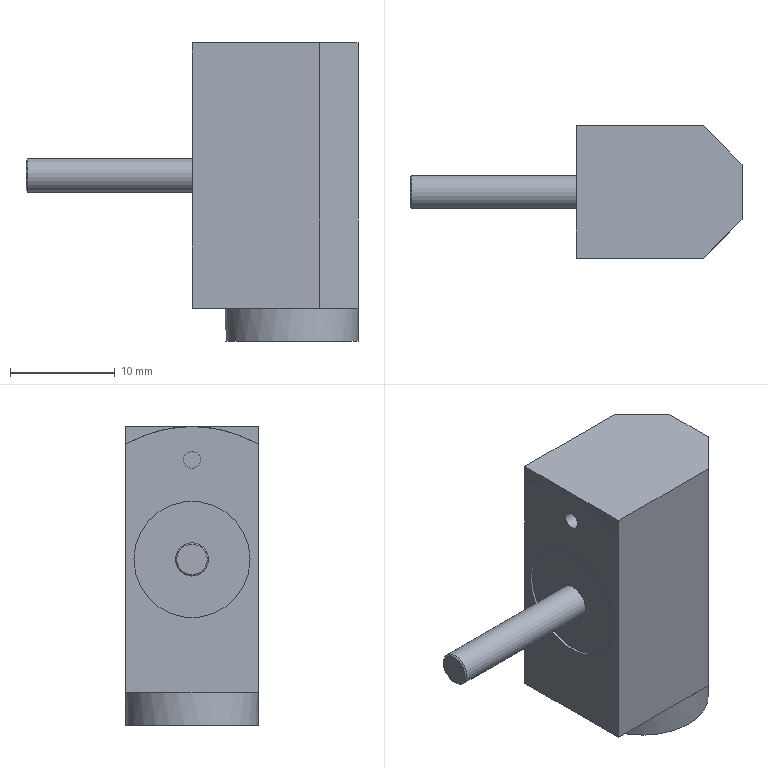Part | NX | features DATUM_CSYS 7, SKETCH 6, EXTRUDE 4, CYLINDER 2, CHAMFER 1, SWP104 1 | 1 solid | 26 faces | box 31.75 x 12.7 x 28.575 mm | volume 3399 mm3 | plane 19 | cylinder 6 | cone 1 | commonest cylinder face diameters 1.587 x1 3.175 x1 9.525 x1 11.113 x1 12.7 x1 25.4 x1
STEP:
#1=CARTESIAN_POINT('',(-9.271,-5.556,15.875));
#2=VERTEX_POINT('',#1);
#3=CARTESIAN_POINT('',(-9.271,0.,15.875));
#4=DIRECTION('',(-1.,0.,0.));
#5=DIRECTION('',(0.,-1.,0.));
#6=AXIS2_PLACEMENT_3D('',#3,#4,#5);
#7=CIRCLE('',#6,5.556);
#8=EDGE_CURVE('',#2,#2,#7,.F.);
#9=ORIENTED_EDGE('',*,*,#8,.F.);
#10=EDGE_LOOP('',(#9));
#11=FACE_BOUND('',#10,.T.);
#12=CARTESIAN_POINT('',(-9.271,0.,17.462));
#13=VERTEX_POINT('',#12);
#14=CARTESIAN_POINT('',(-9.271,0.,15.875));
#15=DIRECTION('',(-1.,0.,0.));
#16=DIRECTION('',(0.,0.,1.));
#17=AXIS2_PLACEMENT_3D('',#14,#15,#16);
#18=CIRCLE('',#17,1.587);
#19=EDGE_CURVE('',#13,#13,#18,.F.);
#20=ORIENTED_EDGE('',*,*,#19,.T.);
#21=EDGE_LOOP('',(#20));
#22=FACE_BOUND('',#21,.T.);
#23=CARTESIAN_POINT('',(-9.271,0.,15.875));
#24=DIRECTION('',(-1.,0.,0.));
#25=DIRECTION('',(0.,0.,1.));
#26=AXIS2_PLACEMENT_3D('',#23,#24,#25);
#27=PLANE('',#26);
#28=ADVANCED_FACE('',(#11,#22),#27,.T.);
#29=CARTESIAN_POINT('',(6.35,0.,0.));
#30=VERTEX_POINT('',#29);
#31=CARTESIAN_POINT('',(0.,0.,0.));
#32=DIRECTION('',(0.,0.,1.));
#33=DIRECTION('',(1.,0.,0.));
#34=AXIS2_PLACEMENT_3D('',#31,#32,#33);
#35=CIRCLE('',#34,6.35);
#36=EDGE_CURVE('',#30,#30,#35,.T.);
#37=ORIENTED_EDGE('',*,*,#36,.T.);
#38=EDGE_LOOP('',(#37));
#39=FACE_BOUND('',#38,.T.);
#40=CARTESIAN_POINT('',(4.49,4.49,3.175));
#41=VERTEX_POINT('',#40);
#42=CARTESIAN_POINT('',(6.35,0.,3.175));
#43=VERTEX_POINT('',#42);
#44=CARTESIAN_POINT('',(0.,0.,3.175));
#45=DIRECTION('',(0.,0.,1.));
#46=DIRECTION('',(1.,0.,0.));
#47=AXIS2_PLACEMENT_3D('',#44,#45,#46);
#48=CIRCLE('',#47,6.35);
#49=EDGE_CURVE('',#41,#43,#48,.F.);
#50=ORIENTED_EDGE('',*,*,#49,.T.);
#51=CARTESIAN_POINT('',(4.49,-4.49,3.175));
#52=VERTEX_POINT('',#51);
#53=CARTESIAN_POINT('',(0.,0.,3.175));
#54=DIRECTION('',(0.,0.,1.));
#55=DIRECTION('',(1.,0.,0.));
#56=AXIS2_PLACEMENT_3D('',#53,#54,#55);
#57=CIRCLE('',#56,6.35);
#58=EDGE_CURVE('',#43,#52,#57,.F.);
#59=ORIENTED_EDGE('',*,*,#58,.T.);
#60=CARTESIAN_POINT('',(0.,-6.35,3.175));
#61=VERTEX_POINT('',#60);
#62=CARTESIAN_POINT('',(0.,0.,3.175));
#63=DIRECTION('',(0.,0.,1.));
#64=DIRECTION('',(1.,0.,0.));
#65=AXIS2_PLACEMENT_3D('',#62,#63,#64);
#66=CIRCLE('',#65,6.35);
#67=EDGE_CURVE('',#52,#61,#66,.F.);
#68=ORIENTED_EDGE('',*,*,#67,.T.);
#69=CARTESIAN_POINT('',(0.,6.35,3.175));
#70=VERTEX_POINT('',#69);
#71=CARTESIAN_POINT('',(0.,0.,3.175));
#72=DIRECTION('',(0.,0.,1.));
#73=DIRECTION('',(1.,0.,0.));
#74=AXIS2_PLACEMENT_3D('',#71,#72,#73);
#75=CIRCLE('',#74,6.35);
#76=EDGE_CURVE('',#61,#70,#75,.F.);
#77=ORIENTED_EDGE('',*,*,#76,.T.);
#78=CARTESIAN_POINT('',(0.,0.,3.175));
#79=DIRECTION('',(0.,0.,1.));
#80=DIRECTION('',(1.,0.,0.));
#81=AXIS2_PLACEMENT_3D('',#78,#79,#80);
#82=CIRCLE('',#81,6.35);
#83=EDGE_CURVE('',#70,#41,#82,.F.);
#84=ORIENTED_EDGE('',*,*,#83,.T.);
#85=EDGE_LOOP('',(#50,#59,#68,#77,#84));
#86=FACE_BOUND('',#85,.T.);
#87=CARTESIAN_POINT('',(0.,0.,0.));
#88=DIRECTION('',(0.,0.,1.));
#89=DIRECTION('',(1.,0.,0.));
#90=AXIS2_PLACEMENT_3D('',#87,#88,#89);
#91=CYLINDRICAL_SURFACE('',#90,6.35);
#92=ADVANCED_FACE('',(#39,#86),#91,.T.);
#93=CARTESIAN_POINT('',(4.763,0.,0.));
#94=VERTEX_POINT('',#93);
#95=CARTESIAN_POINT('',(0.,0.,0.));
#96=DIRECTION('',(0.,0.,1.));
#97=DIRECTION('',(1.,0.,0.));
#98=AXIS2_PLACEMENT_3D('',#95,#96,#97);
#99=CIRCLE('',#98,4.763);
#100=EDGE_CURVE('',#94,#94,#99,.T.);
#101=ORIENTED_EDGE('',*,*,#100,.T.);
#102=EDGE_LOOP('',(#101));
#103=FACE_BOUND('',#102,.T.);
#104=ORIENTED_EDGE('',*,*,#36,.F.);
#105=EDGE_LOOP('',(#104));
#106=FACE_BOUND('',#105,.T.);
#107=CARTESIAN_POINT('',(0.,0.,0.));
#108=DIRECTION('',(0.,0.,-1.));
#109=DIRECTION('',(-1.,0.,0.));
#110=AXIS2_PLACEMENT_3D('',#107,#108,#109);
#111=PLANE('',#110);
#112=ADVANCED_FACE('',(#103,#106),#111,.T.);
#113=CARTESIAN_POINT('',(-9.52,-6.35,28.575));
#114=VERTEX_POINT('',#113);
#115=CARTESIAN_POINT('',(-9.52,-6.35,26.874));
#116=VERTEX_POINT('',#115);
#117=CARTESIAN_POINT('',(-9.52,-6.35,282.892));
#118=DIRECTION('',(0.,0.,-1.));
#119=VECTOR('',#118,1000.);
#120=LINE('',#117,#119);
#121=EDGE_CURVE('',#114,#116,#120,.T.);
#122=ORIENTED_EDGE('',*,*,#121,.T.);
#123=CARTESIAN_POINT('',(-9.525,-6.35,26.874));
#124=VERTEX_POINT('',#123);
#125=CARTESIAN_POINT('',(-9.52,-6.35,26.874));
#126=DIRECTION('',(-1.,0.,0.));
#127=VECTOR('',#126,1000.);
#128=LINE('',#125,#127);
#129=EDGE_CURVE('',#116,#124,#128,.T.);
#130=ORIENTED_EDGE('',*,*,#129,.T.);
#131=CARTESIAN_POINT('',(-9.525,-6.35,3.175));
#132=VERTEX_POINT('',#131);
#133=CARTESIAN_POINT('',(-9.525,-6.35,282.892));
#134=DIRECTION('',(0.,0.,-1.));
#135=VECTOR('',#134,1000.);
#136=LINE('',#133,#135);
#137=EDGE_CURVE('',#124,#132,#136,.T.);
#138=ORIENTED_EDGE('',*,*,#137,.T.);
#139=CARTESIAN_POINT('',(-9.525,-6.35,3.175));
#140=DIRECTION('',(1.,0.,0.));
#141=VECTOR('',#140,1000.);
#142=LINE('',#139,#141);
#143=EDGE_CURVE('',#132,#61,#142,.T.);
#144=ORIENTED_EDGE('',*,*,#143,.T.);
#145=CARTESIAN_POINT('',(2.63,-6.35,3.175));
#146=VERTEX_POINT('',#145);
#147=CARTESIAN_POINT('',(-9.525,-6.35,3.175));
#148=DIRECTION('',(1.,0.,0.));
#149=VECTOR('',#148,1000.);
#150=LINE('',#147,#149);
#151=EDGE_CURVE('',#61,#146,#150,.T.);
#152=ORIENTED_EDGE('',*,*,#151,.T.);
#153=CARTESIAN_POINT('',(2.63,-6.35,28.575));
#154=VERTEX_POINT('',#153);
#155=CARTESIAN_POINT('',(2.63,-6.35,282.892));
#156=DIRECTION('',(0.,0.,-1.));
#157=VECTOR('',#156,1000.);
#158=LINE('',#155,#157);
#159=EDGE_CURVE('',#154,#146,#158,.T.);
#160=ORIENTED_EDGE('',*,*,#159,.F.);
#161=CARTESIAN_POINT('',(-9.525,-6.35,28.575));
#162=DIRECTION('',(1.,0.,0.));
#163=VECTOR('',#162,1000.);
#164=LINE('',#161,#163);
#165=EDGE_CURVE('',#114,#154,#164,.T.);
#166=ORIENTED_EDGE('',*,*,#165,.F.);
#167=EDGE_LOOP('',(#122,#130,#138,#144,#152,#160,#166));
#168=FACE_BOUND('',#167,.T.);
#169=CARTESIAN_POINT('',(-9.525,-6.35,282.892));
#170=DIRECTION('',(0.,1.,0.));
#171=DIRECTION('',(-1.,0.,0.));
#172=AXIS2_PLACEMENT_3D('',#169,#170,#171);
#173=PLANE('',#172);
#174=ADVANCED_FACE('',(#168),#173,.F.);
#175=CARTESIAN_POINT('',(6.35,-2.63,28.575));
#176=VERTEX_POINT('',#175);
#177=CARTESIAN_POINT('',(2.63,-6.35,28.575));
#178=DIRECTION('',(0.7071,0.7071,0.));
#179=VECTOR('',#178,1000.);
#180=LINE('',#177,#179);
#181=EDGE_CURVE('',#154,#176,#180,.T.);
#182=ORIENTED_EDGE('',*,*,#181,.F.);
#183=ORIENTED_EDGE('',*,*,#159,.T.);
#184=CARTESIAN_POINT('',(2.63,-6.35,3.175));
#185=DIRECTION('',(0.7071,0.7071,0.));
#186=VECTOR('',#185,1000.);
#187=LINE('',#184,#186);
#188=EDGE_CURVE('',#146,#52,#187,.T.);
#189=ORIENTED_EDGE('',*,*,#188,.T.);
#190=CARTESIAN_POINT('',(6.35,-2.63,3.175));
#191=VERTEX_POINT('',#190);
#192=CARTESIAN_POINT('',(2.63,-6.35,3.175));
#193=DIRECTION('',(0.7071,0.7071,0.));
#194=VECTOR('',#193,1000.);
#195=LINE('',#192,#194);
#196=EDGE_CURVE('',#52,#191,#195,.T.);
#197=ORIENTED_EDGE('',*,*,#196,.T.);
#198=CARTESIAN_POINT('',(6.35,-2.63,282.892));
#199=DIRECTION('',(0.,0.,-1.));
#200=VECTOR('',#199,1000.);
#201=LINE('',#198,#200);
#202=EDGE_CURVE('',#176,#191,#201,.T.);
#203=ORIENTED_EDGE('',*,*,#202,.F.);
#204=EDGE_LOOP('',(#182,#183,#189,#197,#203));
#205=FACE_BOUND('',#204,.T.);
#206=CARTESIAN_POINT('',(2.63,-6.35,282.892));
#207=DIRECTION('',(-0.7071,0.7071,0.));
#208=DIRECTION('',(-0.7071,-0.7071,0.));
#209=AXIS2_PLACEMENT_3D('',#206,#207,#208);
#210=PLANE('',#209);
#211=ADVANCED_FACE('',(#205),#210,.F.);
#212=CARTESIAN_POINT('',(6.35,2.63,28.575));
#213=VERTEX_POINT('',#212);
#214=CARTESIAN_POINT('',(6.35,2.63,3.175));
#215=VERTEX_POINT('',#214);
#216=CARTESIAN_POINT('',(6.35,2.63,282.892));
#217=DIRECTION('',(0.,0.,-1.));
#218=VECTOR('',#217,1000.);
#219=LINE('',#216,#218);
#220=EDGE_CURVE('',#213,#215,#219,.T.);
#221=ORIENTED_EDGE('',*,*,#220,.F.);
#222=CARTESIAN_POINT('',(6.35,-2.63,28.575));
#223=DIRECTION('',(0.,1.,0.));
#224=VECTOR('',#223,1000.);
#225=LINE('',#222,#224);
#226=EDGE_CURVE('',#176,#213,#225,.T.);
#227=ORIENTED_EDGE('',*,*,#226,.F.);
#228=ORIENTED_EDGE('',*,*,#202,.T.);
#229=CARTESIAN_POINT('',(6.35,-2.63,3.175));
#230=DIRECTION('',(0.,1.,0.));
#231=VECTOR('',#230,1000.);
#232=LINE('',#229,#231);
#233=EDGE_CURVE('',#191,#43,#232,.T.);
#234=ORIENTED_EDGE('',*,*,#233,.T.);
#235=CARTESIAN_POINT('',(6.35,-2.63,3.175));
#236=DIRECTION('',(0.,1.,0.));
#237=VECTOR('',#236,1000.);
#238=LINE('',#235,#237);
#239=EDGE_CURVE('',#43,#215,#238,.T.);
#240=ORIENTED_EDGE('',*,*,#239,.T.);
#241=EDGE_LOOP('',(#221,#227,#228,#234,#240));
#242=FACE_BOUND('',#241,.T.);
#243=CARTESIAN_POINT('',(6.35,-2.63,282.892));
#244=DIRECTION('',(-1.,0.,0.));
#245=DIRECTION('',(0.,-1.,0.));
#246=AXIS2_PLACEMENT_3D('',#243,#244,#245);
#247=PLANE('',#246);
#248=ADVANCED_FACE('',(#242),#247,.F.);
#249=CARTESIAN_POINT('',(2.63,6.35,28.575));
#250=VERTEX_POINT('',#249);
#251=CARTESIAN_POINT('',(6.35,2.63,28.575));
#252=DIRECTION('',(-0.7071,0.7071,0.));
#253=VECTOR('',#252,1000.);
#254=LINE('',#251,#253);
#255=EDGE_CURVE('',#213,#250,#254,.T.);
#256=ORIENTED_EDGE('',*,*,#255,.F.);
#257=ORIENTED_EDGE('',*,*,#220,.T.);
#258=CARTESIAN_POINT('',(6.35,2.63,3.175));
#259=DIRECTION('',(-0.7071,0.7071,0.));
#260=VECTOR('',#259,1000.);
#261=LINE('',#258,#260);
#262=EDGE_CURVE('',#215,#41,#261,.T.);
#263=ORIENTED_EDGE('',*,*,#262,.T.);
#264=CARTESIAN_POINT('',(2.63,6.35,3.175));
#265=VERTEX_POINT('',#264);
#266=CARTESIAN_POINT('',(6.35,2.63,3.175));
#267=DIRECTION('',(-0.7071,0.7071,0.));
#268=VECTOR('',#267,1000.);
#269=LINE('',#266,#268);
#270=EDGE_CURVE('',#41,#265,#269,.T.);
#271=ORIENTED_EDGE('',*,*,#270,.T.);
#272=CARTESIAN_POINT('',(2.63,6.35,282.892));
#273=DIRECTION('',(0.,0.,-1.));
#274=VECTOR('',#273,1000.);
#275=LINE('',#272,#274);
#276=EDGE_CURVE('',#250,#265,#275,.T.);
#277=ORIENTED_EDGE('',*,*,#276,.F.);
#278=EDGE_LOOP('',(#256,#257,#263,#271,#277));
#279=FACE_BOUND('',#278,.T.);
#280=CARTESIAN_POINT('',(6.35,2.63,282.892));
#281=DIRECTION('',(-0.7071,-0.7071,0.));
#282=DIRECTION('',(0.7071,-0.7071,0.));
#283=AXIS2_PLACEMENT_3D('',#280,#281,#282);
#284=PLANE('',#283);
#285=ADVANCED_FACE('',(#279),#284,.F.);
#286=CARTESIAN_POINT('',(-9.525,6.35,26.874));
#287=VERTEX_POINT('',#286);
#288=CARTESIAN_POINT('',(-9.525,6.35,3.175));
#289=VERTEX_POINT('',#288);
#290=CARTESIAN_POINT('',(-9.525,6.35,282.892));
#291=DIRECTION('',(0.,0.,-1.));
#292=VECTOR('',#291,1000.);
#293=LINE('',#290,#292);
#294=EDGE_CURVE('',#287,#289,#293,.T.);
#295=ORIENTED_EDGE('',*,*,#294,.F.);
#296=CARTESIAN_POINT('',(-9.52,6.35,26.874));
#297=VERTEX_POINT('',#296);
#298=CARTESIAN_POINT('',(-9.52,6.35,26.874));
#299=DIRECTION('',(-1.,0.,0.));
#300=VECTOR('',#299,1000.);
#301=LINE('',#298,#300);
#302=EDGE_CURVE('',#287,#297,#301,.F.);
#303=ORIENTED_EDGE('',*,*,#302,.T.);
#304=CARTESIAN_POINT('',(-9.52,6.35,28.575));
#305=VERTEX_POINT('',#304);
#306=CARTESIAN_POINT('',(-9.52,6.35,282.892));
#307=DIRECTION('',(0.,0.,1.));
#308=VECTOR('',#307,1000.);
#309=LINE('',#306,#308);
#310=EDGE_CURVE('',#297,#305,#309,.T.);
#311=ORIENTED_EDGE('',*,*,#310,.T.);
#312=CARTESIAN_POINT('',(2.63,6.35,28.575));
#313=DIRECTION('',(-1.,0.,0.));
#314=VECTOR('',#313,1000.);
#315=LINE('',#312,#314);
#316=EDGE_CURVE('',#250,#305,#315,.T.);
#317=ORIENTED_EDGE('',*,*,#316,.F.);
#318=ORIENTED_EDGE('',*,*,#276,.T.);
#319=CARTESIAN_POINT('',(2.63,6.35,3.175));
#320=DIRECTION('',(-1.,0.,0.));
#321=VECTOR('',#320,1000.);
#322=LINE('',#319,#321);
#323=EDGE_CURVE('',#265,#70,#322,.T.);
#324=ORIENTED_EDGE('',*,*,#323,.T.);
#325=CARTESIAN_POINT('',(2.63,6.35,3.175));
#326=DIRECTION('',(-1.,0.,0.));
#327=VECTOR('',#326,1000.);
#328=LINE('',#325,#327);
#329=EDGE_CURVE('',#70,#289,#328,.T.);
#330=ORIENTED_EDGE('',*,*,#329,.T.);
#331=EDGE_LOOP('',(#295,#303,#311,#317,#318,#324,#330));
#332=FACE_BOUND('',#331,.T.);
#333=CARTESIAN_POINT('',(2.63,6.35,282.892));
#334=DIRECTION('',(0.,-1.,0.));
#335=DIRECTION('',(0.,0.,-1.));
#336=AXIS2_PLACEMENT_3D('',#333,#334,#335);
#337=PLANE('',#336);
#338=ADVANCED_FACE('',(#332),#337,.F.);
#339=ORIENTED_EDGE('',*,*,#58,.F.);
#340=ORIENTED_EDGE('',*,*,#233,.F.);
#341=ORIENTED_EDGE('',*,*,#196,.F.);
#342=EDGE_LOOP('',(#339,#340,#341));
#343=FACE_BOUND('',#342,.T.);
#344=CARTESIAN_POINT('',(0.,0.,3.175));
#345=DIRECTION('',(0.,0.,1.));
#346=DIRECTION('',(1.,0.,0.));
#347=AXIS2_PLACEMENT_3D('',#344,#345,#346);
#348=PLANE('',#347);
#349=ADVANCED_FACE('',(#343),#348,.F.);
#350=ORIENTED_EDGE('',*,*,#67,.F.);
#351=ORIENTED_EDGE('',*,*,#188,.F.);
#352=ORIENTED_EDGE('',*,*,#151,.F.);
#353=EDGE_LOOP('',(#350,#351,#352));
#354=FACE_BOUND('',#353,.T.);
#355=CARTESIAN_POINT('',(0.,0.,3.175));
#356=DIRECTION('',(0.,0.,1.));
#357=DIRECTION('',(1.,0.,0.));
#358=AXIS2_PLACEMENT_3D('',#355,#356,#357);
#359=PLANE('',#358);
#360=ADVANCED_FACE('',(#354),#359,.F.);
#361=ORIENTED_EDGE('',*,*,#76,.F.);
#362=ORIENTED_EDGE('',*,*,#143,.F.);
#363=CARTESIAN_POINT('',(-9.525,6.35,3.175));
#364=DIRECTION('',(0.,-1.,0.));
#365=VECTOR('',#364,1000.);
#366=LINE('',#363,#365);
#367=EDGE_CURVE('',#289,#132,#366,.T.);
#368=ORIENTED_EDGE('',*,*,#367,.F.);
#369=ORIENTED_EDGE('',*,*,#329,.F.);
#370=EDGE_LOOP('',(#361,#362,#368,#369));
#371=FACE_BOUND('',#370,.T.);
#372=CARTESIAN_POINT('',(0.,0.,3.175));
#373=DIRECTION('',(0.,0.,1.));
#374=DIRECTION('',(1.,0.,0.));
#375=AXIS2_PLACEMENT_3D('',#372,#373,#374);
#376=PLANE('',#375);
#377=ADVANCED_FACE('',(#371),#376,.F.);
#378=ORIENTED_EDGE('',*,*,#83,.F.);
#379=ORIENTED_EDGE('',*,*,#323,.F.);
#380=ORIENTED_EDGE('',*,*,#270,.F.);
#381=EDGE_LOOP('',(#378,#379,#380));
#382=FACE_BOUND('',#381,.T.);
#383=CARTESIAN_POINT('',(0.,0.,3.175));
#384=DIRECTION('',(0.,0.,1.));
#385=DIRECTION('',(1.,0.,0.));
#386=AXIS2_PLACEMENT_3D('',#383,#384,#385);
#387=PLANE('',#386);
#388=ADVANCED_FACE('',(#382),#387,.F.);
#389=CARTESIAN_POINT('',(-9.525,-5.556,15.875));
#390=VERTEX_POINT('',#389);
#391=CARTESIAN_POINT('',(-9.525,0.,15.875));
#392=DIRECTION('',(-1.,0.,0.));
#393=DIRECTION('',(0.,-1.,0.));
#394=AXIS2_PLACEMENT_3D('',#391,#392,#393);
#395=CIRCLE('',#394,5.556);
#396=EDGE_CURVE('',#390,#390,#395,.T.);
#397=ORIENTED_EDGE('',*,*,#396,.F.);
#398=EDGE_LOOP('',(#397));
#399=FACE_BOUND('',#398,.T.);
#400=CARTESIAN_POINT('',(-9.525,-0.7937,25.4));
#401=VERTEX_POINT('',#400);
#402=CARTESIAN_POINT('',(-9.525,0.,25.4));
#403=DIRECTION('',(-1.,0.,0.));
#404=DIRECTION('',(0.,-1.,0.));
#405=AXIS2_PLACEMENT_3D('',#402,#403,#404);
#406=CIRCLE('',#405,0.7937);
#407=EDGE_CURVE('',#401,#401,#406,.T.);
#408=ORIENTED_EDGE('',*,*,#407,.F.);
#409=EDGE_LOOP('',(#408));
#410=FACE_BOUND('',#409,.T.);
#411=CARTESIAN_POINT('',(-9.525,0.,15.875));
#412=DIRECTION('',(1.,0.,0.));
#413=DIRECTION('',(0.,-1.,0.));
#414=AXIS2_PLACEMENT_3D('',#411,#412,#413);
#415=CIRCLE('',#414,12.7);
#416=EDGE_CURVE('',#287,#124,#415,.T.);
#417=ORIENTED_EDGE('',*,*,#416,.F.);
#418=ORIENTED_EDGE('',*,*,#294,.T.);
#419=ORIENTED_EDGE('',*,*,#367,.T.);
#420=ORIENTED_EDGE('',*,*,#137,.F.);
#421=EDGE_LOOP('',(#417,#418,#419,#420));
#422=FACE_BOUND('',#421,.T.);
#423=CARTESIAN_POINT('',(-9.525,6.35,282.892));
#424=DIRECTION('',(1.,0.,0.));
#425=DIRECTION('',(0.,1.,0.));
#426=AXIS2_PLACEMENT_3D('',#423,#424,#425);
#427=PLANE('',#426);
#428=ADVANCED_FACE('',(#399,#410,#422),#427,.F.);
#429=ORIENTED_EDGE('',*,*,#49,.F.);
#430=ORIENTED_EDGE('',*,*,#262,.F.);
#431=ORIENTED_EDGE('',*,*,#239,.F.);
#432=EDGE_LOOP('',(#429,#430,#431));
#433=FACE_BOUND('',#432,.T.);
#434=CARTESIAN_POINT('',(0.,0.,3.175));
#435=DIRECTION('',(0.,0.,1.));
#436=DIRECTION('',(1.,0.,0.));
#437=AXIS2_PLACEMENT_3D('',#434,#435,#436);
#438=PLANE('',#437);
#439=ADVANCED_FACE('',(#433),#438,.F.);
#440=CARTESIAN_POINT('',(-9.52,0.,28.575));
#441=VERTEX_POINT('',#440);
#442=CARTESIAN_POINT('',(-9.52,0.,28.575));
#443=DIRECTION('',(0.,1.,0.));
#444=VECTOR('',#443,1000.);
#445=LINE('',#442,#444);
#446=EDGE_CURVE('',#114,#441,#445,.T.);
#447=ORIENTED_EDGE('',*,*,#446,.F.);
#448=ORIENTED_EDGE('',*,*,#165,.T.);
#449=ORIENTED_EDGE('',*,*,#181,.T.);
#450=ORIENTED_EDGE('',*,*,#226,.T.);
#451=ORIENTED_EDGE('',*,*,#255,.T.);
#452=ORIENTED_EDGE('',*,*,#316,.T.);
#453=CARTESIAN_POINT('',(-9.52,0.,28.575));
#454=DIRECTION('',(0.,1.,0.));
#455=VECTOR('',#454,1000.);
#456=LINE('',#453,#455);
#457=EDGE_CURVE('',#441,#305,#456,.T.);
#458=ORIENTED_EDGE('',*,*,#457,.F.);
#459=EDGE_LOOP('',(#447,#448,#449,#450,#451,#452,#458));
#460=FACE_BOUND('',#459,.T.);
#461=CARTESIAN_POINT('',(0.,0.,28.575));
#462=DIRECTION('',(0.,0.,1.));
#463=DIRECTION('',(1.,0.,0.));
#464=AXIS2_PLACEMENT_3D('',#461,#462,#463);
#465=PLANE('',#464);
#466=ADVANCED_FACE('',(#460),#465,.T.);
#467=CARTESIAN_POINT('',(-9.52,0.,15.875));
#468=DIRECTION('',(1.,0.,0.));
#469=DIRECTION('',(0.,-1.,0.));
#470=AXIS2_PLACEMENT_3D('',#467,#468,#469);
#471=CIRCLE('',#470,12.7);
#472=EDGE_CURVE('',#116,#441,#471,.F.);
#473=ORIENTED_EDGE('',*,*,#472,.T.);
#474=CARTESIAN_POINT('',(-9.52,0.,15.875));
#475=DIRECTION('',(1.,0.,0.));
#476=DIRECTION('',(0.,-1.,0.));
#477=AXIS2_PLACEMENT_3D('',#474,#475,#476);
#478=CIRCLE('',#477,12.7);
#479=EDGE_CURVE('',#441,#297,#478,.F.);
#480=ORIENTED_EDGE('',*,*,#479,.T.);
#481=ORIENTED_EDGE('',*,*,#302,.F.);
#482=ORIENTED_EDGE('',*,*,#416,.T.);
#483=ORIENTED_EDGE('',*,*,#129,.F.);
#484=EDGE_LOOP('',(#473,#480,#481,#482,#483));
#485=FACE_BOUND('',#484,.T.);
#486=CARTESIAN_POINT('',(-9.52,0.,15.875));
#487=DIRECTION('',(-1.,0.,0.));
#488=DIRECTION('',(0.,0.,1.));
#489=AXIS2_PLACEMENT_3D('',#486,#487,#488);
#490=CYLINDRICAL_SURFACE('',#489,12.7);
#491=ADVANCED_FACE('',(#485),#490,.T.);
#492=ORIENTED_EDGE('',*,*,#446,.T.);
#493=ORIENTED_EDGE('',*,*,#472,.F.);
#494=ORIENTED_EDGE('',*,*,#121,.F.);
#495=EDGE_LOOP('',(#492,#493,#494));
#496=FACE_BOUND('',#495,.T.);
#497=CARTESIAN_POINT('',(-9.52,0.,15.875));
#498=DIRECTION('',(1.,0.,0.));
#499=DIRECTION('',(0.,0.,-1.));
#500=AXIS2_PLACEMENT_3D('',#497,#498,#499);
#501=PLANE('',#500);
#502=ADVANCED_FACE('',(#496),#501,.F.);
#503=ORIENTED_EDGE('',*,*,#479,.F.);
#504=ORIENTED_EDGE('',*,*,#457,.T.);
#505=ORIENTED_EDGE('',*,*,#310,.F.);
#506=EDGE_LOOP('',(#503,#504,#505));
#507=FACE_BOUND('',#506,.T.);
#508=CARTESIAN_POINT('',(-9.52,0.,15.875));
#509=DIRECTION('',(1.,0.,0.));
#510=DIRECTION('',(0.,0.,-1.));
#511=AXIS2_PLACEMENT_3D('',#508,#509,#510);
#512=PLANE('',#511);
#513=ADVANCED_FACE('',(#507),#512,.F.);
#514=CARTESIAN_POINT('',(-4.953,-0.7937,25.4));
#515=VERTEX_POINT('',#514);
#516=CARTESIAN_POINT('',(-4.953,0.,25.4));
#517=DIRECTION('',(-1.,0.,0.));
#518=DIRECTION('',(0.,-1.,0.));
#519=AXIS2_PLACEMENT_3D('',#516,#517,#518);
#520=CIRCLE('',#519,0.7937);
#521=EDGE_CURVE('',#515,#515,#520,.F.);
#522=ORIENTED_EDGE('',*,*,#521,.T.);
#523=EDGE_LOOP('',(#522));
#524=FACE_BOUND('',#523,.T.);
#525=ORIENTED_EDGE('',*,*,#407,.T.);
#526=EDGE_LOOP('',(#525));
#527=FACE_BOUND('',#526,.T.);
#528=CARTESIAN_POINT('',(-4.953,0.,25.4));
#529=DIRECTION('',(-1.,0.,0.));
#530=DIRECTION('',(0.,-1.,0.));
#531=AXIS2_PLACEMENT_3D('',#528,#529,#530);
#532=CYLINDRICAL_SURFACE('',#531,0.7937);
#533=ADVANCED_FACE('',(#524,#527),#532,.F.);
#534=ORIENTED_EDGE('',*,*,#521,.F.);
#535=EDGE_LOOP('',(#534));
#536=FACE_BOUND('',#535,.T.);
#537=CARTESIAN_POINT('',(-4.953,0.,25.4));
#538=DIRECTION('',(-1.,0.,0.));
#539=DIRECTION('',(0.,0.,1.));
#540=AXIS2_PLACEMENT_3D('',#537,#538,#539);
#541=PLANE('',#540);
#542=ADVANCED_FACE('',(#536),#541,.T.);
#543=ORIENTED_EDGE('',*,*,#8,.T.);
#544=EDGE_LOOP('',(#543));
#545=FACE_BOUND('',#544,.T.);
#546=ORIENTED_EDGE('',*,*,#396,.T.);
#547=EDGE_LOOP('',(#546));
#548=FACE_BOUND('',#547,.T.);
#549=CARTESIAN_POINT('',(-9.271,0.,15.875));
#550=DIRECTION('',(-1.,0.,0.));
#551=DIRECTION('',(0.,0.,1.));
#552=AXIS2_PLACEMENT_3D('',#549,#550,#551);
#553=CYLINDRICAL_SURFACE('',#552,5.556);
#554=ADVANCED_FACE('',(#545,#548),#553,.F.);
#555=CARTESIAN_POINT('',(-25.273,0.,17.462));
#556=VERTEX_POINT('',#555);
#557=CARTESIAN_POINT('',(-25.273,0.,15.875));
#558=DIRECTION('',(-1.,0.,0.));
#559=DIRECTION('',(0.,0.,1.));
#560=AXIS2_PLACEMENT_3D('',#557,#558,#559);
#561=CIRCLE('',#560,1.587);
#562=EDGE_CURVE('',#556,#556,#561,.F.);
#563=ORIENTED_EDGE('',*,*,#562,.T.);
#564=EDGE_LOOP('',(#563));
#565=FACE_BOUND('',#564,.T.);
#566=ORIENTED_EDGE('',*,*,#19,.F.);
#567=EDGE_LOOP('',(#566));
#568=FACE_BOUND('',#567,.T.);
#569=CARTESIAN_POINT('',(-25.4,0.,15.875));
#570=DIRECTION('',(1.,0.,0.));
#571=DIRECTION('',(0.,0.,-1.));
#572=AXIS2_PLACEMENT_3D('',#569,#570,#571);
#573=CYLINDRICAL_SURFACE('',#572,1.587);
#574=ADVANCED_FACE('',(#565,#568),#573,.T.);
#575=CARTESIAN_POINT('',(-25.4,0.,17.335));
#576=VERTEX_POINT('',#575);
#577=CARTESIAN_POINT('',(-25.4,0.,15.875));
#578=DIRECTION('',(-1.,0.,0.));
#579=DIRECTION('',(0.,0.,1.));
#580=AXIS2_PLACEMENT_3D('',#577,#578,#579);
#581=CIRCLE('',#580,1.46);
#582=EDGE_CURVE('',#576,#576,#581,.T.);
#583=ORIENTED_EDGE('',*,*,#582,.T.);
#584=EDGE_LOOP('',(#583));
#585=FACE_BOUND('',#584,.T.);
#586=CARTESIAN_POINT('',(-25.4,0.,15.875));
#587=DIRECTION('',(-1.,0.,0.));
#588=DIRECTION('',(0.,0.,1.));
#589=AXIS2_PLACEMENT_3D('',#586,#587,#588);
#590=PLANE('',#589);
#591=ADVANCED_FACE('',(#585),#590,.T.);
#592=ORIENTED_EDGE('',*,*,#562,.F.);
#593=EDGE_LOOP('',(#592));
#594=FACE_BOUND('',#593,.T.);
#595=ORIENTED_EDGE('',*,*,#582,.F.);
#596=EDGE_LOOP('',(#595));
#597=FACE_BOUND('',#596,.T.);
#598=CARTESIAN_POINT('',(-25.4,0.,15.875));
#599=DIRECTION('',(1.,0.,0.));
#600=DIRECTION('',(0.,0.,-1.));
#601=AXIS2_PLACEMENT_3D('',#598,#599,#600);
#602=CONICAL_SURFACE('',#601,1.46,0.7854);
#603=ADVANCED_FACE('',(#594,#597),#602,.T.);
#604=CARTESIAN_POINT('',(4.763,0.,26.194));
#605=VERTEX_POINT('',#604);
#606=CARTESIAN_POINT('',(0.,0.,26.194));
#607=DIRECTION('',(0.,0.,-1.));
#608=DIRECTION('',(1.,0.,0.));
#609=AXIS2_PLACEMENT_3D('',#606,#607,#608);
#610=CIRCLE('',#609,4.763);
#611=EDGE_CURVE('',#605,#605,#610,.F.);
#612=ORIENTED_EDGE('',*,*,#611,.F.);
#613=EDGE_LOOP('',(#612));
#614=FACE_BOUND('',#613,.T.);
#615=CARTESIAN_POINT('',(0.,0.,26.194));
#616=DIRECTION('',(0.,0.,1.));
#617=DIRECTION('',(1.,0.,0.));
#618=AXIS2_PLACEMENT_3D('',#615,#616,#617);
#619=PLANE('',#618);
#620=ADVANCED_FACE('',(#614),#619,.F.);
#621=ORIENTED_EDGE('',*,*,#611,.T.);
#622=EDGE_LOOP('',(#621));
#623=FACE_BOUND('',#622,.T.);
#624=ORIENTED_EDGE('',*,*,#100,.F.);
#625=EDGE_LOOP('',(#624));
#626=FACE_BOUND('',#625,.T.);
#627=CARTESIAN_POINT('',(0.,0.,0.));
#628=DIRECTION('',(0.,0.,1.));
#629=DIRECTION('',(1.,0.,0.));
#630=AXIS2_PLACEMENT_3D('',#627,#628,#629);
#631=CYLINDRICAL_SURFACE('',#630,4.763);
#632=ADVANCED_FACE('',(#623,#626),#631,.F.);
#633=CLOSED_SHELL('',(#28,#92,#112,#174,#211,#248,#285,#338,#349,#360,#377,#388,#428,#439,#466,#491,#502,#513,#533,#542,#554,#574,#591,#603,#620,#632));
#634=MANIFOLD_SOLID_BREP('',#633);
#635=(LENGTH_UNIT()NAMED_UNIT(*)SI_UNIT(.MILLI.,.METRE.));
#636=UNCERTAINTY_MEASURE_WITH_UNIT(LENGTH_MEASURE(0.00001),#635,'','');
#637=(NAMED_UNIT(*)PLANE_ANGLE_UNIT()SI_UNIT($,.RADIAN.));
#638=(NAMED_UNIT(*)SI_UNIT($,.STERADIAN.)SOLID_ANGLE_UNIT());
#639=(GEOMETRIC_REPRESENTATION_CONTEXT(3)GLOBAL_UNCERTAINTY_ASSIGNED_CONTEXT((#636))GLOBAL_UNIT_ASSIGNED_CONTEXT((#635,#637,#638))REPRESENTATION_CONTEXT('',''));
#640=ADVANCED_BREP_SHAPE_REPRESENTATION('',(#634),#639);